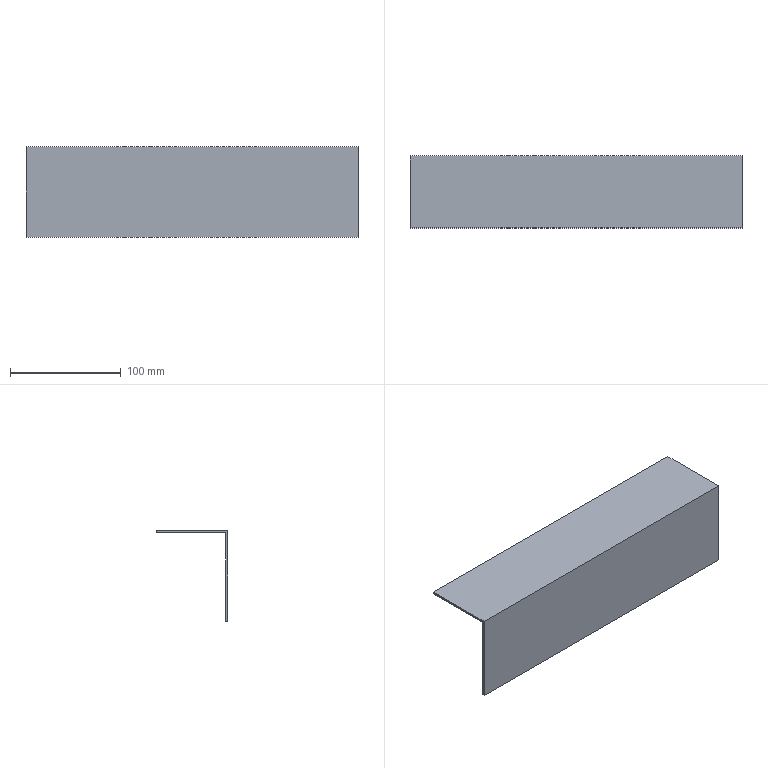Part | STEP file | MYT-A01-P21 | 1 solid | 8 faces | box 300 x 65 x 82 mm | volume 87000 mm3 | plane 8
STEP:
#1=CARTESIAN_POINT('',(-150.,-30.5,0.));
#2=VERTEX_POINT('',#1);
#3=CARTESIAN_POINT('',(150.,-30.5,0.));
#4=VERTEX_POINT('',#3);
#5=CARTESIAN_POINT('',(150.,-30.5,0.));
#6=DIRECTION('',(1.,0.,0.));
#7=VECTOR('',#6,1000.);
#8=LINE('',#5,#7);
#9=EDGE_CURVE('',#2,#4,#8,.T.);
#10=ORIENTED_EDGE('',*,*,#9,.F.);
#11=CARTESIAN_POINT('',(-150.,32.5,0.));
#12=VERTEX_POINT('',#11);
#13=CARTESIAN_POINT('',(-150.,32.5,0.));
#14=DIRECTION('',(0.,-1.,0.));
#15=VECTOR('',#14,1000.);
#16=LINE('',#13,#15);
#17=EDGE_CURVE('',#12,#2,#16,.T.);
#18=ORIENTED_EDGE('',*,*,#17,.F.);
#19=CARTESIAN_POINT('',(150.,32.5,0.));
#20=VERTEX_POINT('',#19);
#21=CARTESIAN_POINT('',(-150.,32.5,0.));
#22=DIRECTION('',(-1.,0.,0.));
#23=VECTOR('',#22,1000.);
#24=LINE('',#21,#23);
#25=EDGE_CURVE('',#20,#12,#24,.T.);
#26=ORIENTED_EDGE('',*,*,#25,.F.);
#27=CARTESIAN_POINT('',(150.,32.5,0.));
#28=DIRECTION('',(0.,1.,0.));
#29=VECTOR('',#28,1000.);
#30=LINE('',#27,#29);
#31=EDGE_CURVE('',#4,#20,#30,.T.);
#32=ORIENTED_EDGE('',*,*,#31,.F.);
#33=EDGE_LOOP('',(#10,#18,#26,#32));
#34=FACE_OUTER_BOUND('',#33,.T.);
#35=CARTESIAN_POINT('',(0.,0.,0.));
#36=DIRECTION('',(0.,0.,1.));
#37=DIRECTION('',(1.,0.,0.));
#38=AXIS2_PLACEMENT_3D('',#35,#36,#37);
#39=PLANE('',#38);
#40=ADVANCED_FACE('',(#34),#39,.F.);
#41=CARTESIAN_POINT('',(150.,-32.5,2.));
#42=VERTEX_POINT('',#41);
#43=CARTESIAN_POINT('',(150.,-32.5,-80.));
#44=VERTEX_POINT('',#43);
#45=CARTESIAN_POINT('',(150.,-32.5,2.));
#46=DIRECTION('',(0.,0.,-1.));
#47=VECTOR('',#46,1000.);
#48=LINE('',#45,#47);
#49=EDGE_CURVE('',#42,#44,#48,.T.);
#50=ORIENTED_EDGE('',*,*,#49,.T.);
#51=CARTESIAN_POINT('',(150.,-30.5,-80.));
#52=VERTEX_POINT('',#51);
#53=CARTESIAN_POINT('',(150.,-32.5,-80.));
#54=DIRECTION('',(0.,-1.,0.));
#55=VECTOR('',#54,1000.);
#56=LINE('',#53,#55);
#57=EDGE_CURVE('',#52,#44,#56,.T.);
#58=ORIENTED_EDGE('',*,*,#57,.F.);
#59=CARTESIAN_POINT('',(150.,-30.5,-80.));
#60=DIRECTION('',(0.,0.,1.));
#61=VECTOR('',#60,1000.);
#62=LINE('',#59,#61);
#63=EDGE_CURVE('',#52,#4,#62,.T.);
#64=ORIENTED_EDGE('',*,*,#63,.T.);
#65=ORIENTED_EDGE('',*,*,#31,.T.);
#66=CARTESIAN_POINT('',(150.,32.5,2.));
#67=VERTEX_POINT('',#66);
#68=CARTESIAN_POINT('',(150.,32.5,2.));
#69=DIRECTION('',(0.,0.,-1.));
#70=VECTOR('',#69,1000.);
#71=LINE('',#68,#70);
#72=EDGE_CURVE('',#67,#20,#71,.T.);
#73=ORIENTED_EDGE('',*,*,#72,.F.);
#74=CARTESIAN_POINT('',(150.,32.5,2.));
#75=DIRECTION('',(0.,1.,0.));
#76=VECTOR('',#75,1000.);
#77=LINE('',#74,#76);
#78=EDGE_CURVE('',#42,#67,#77,.T.);
#79=ORIENTED_EDGE('',*,*,#78,.F.);
#80=EDGE_LOOP('',(#50,#58,#64,#65,#73,#79));
#81=FACE_OUTER_BOUND('',#80,.T.);
#82=CARTESIAN_POINT('',(150.,32.5,2.));
#83=DIRECTION('',(-1.,0.,0.));
#84=DIRECTION('',(0.,0.,1.));
#85=AXIS2_PLACEMENT_3D('',#82,#83,#84);
#86=PLANE('',#85);
#87=ADVANCED_FACE('',(#81),#86,.F.);
#88=ORIENTED_EDGE('',*,*,#25,.T.);
#89=CARTESIAN_POINT('',(-150.,32.5,2.));
#90=VERTEX_POINT('',#89);
#91=CARTESIAN_POINT('',(-150.,32.5,2.));
#92=DIRECTION('',(0.,0.,-1.));
#93=VECTOR('',#92,1000.);
#94=LINE('',#91,#93);
#95=EDGE_CURVE('',#90,#12,#94,.T.);
#96=ORIENTED_EDGE('',*,*,#95,.F.);
#97=CARTESIAN_POINT('',(-150.,32.5,2.));
#98=DIRECTION('',(-1.,0.,0.));
#99=VECTOR('',#98,1000.);
#100=LINE('',#97,#99);
#101=EDGE_CURVE('',#67,#90,#100,.T.);
#102=ORIENTED_EDGE('',*,*,#101,.F.);
#103=ORIENTED_EDGE('',*,*,#72,.T.);
#104=EDGE_LOOP('',(#88,#96,#102,#103));
#105=FACE_OUTER_BOUND('',#104,.T.);
#106=CARTESIAN_POINT('',(-150.,32.5,2.));
#107=DIRECTION('',(0.,-1.,0.));
#108=DIRECTION('',(0.,0.,-1.));
#109=AXIS2_PLACEMENT_3D('',#106,#107,#108);
#110=PLANE('',#109);
#111=ADVANCED_FACE('',(#105),#110,.F.);
#112=ORIENTED_EDGE('',*,*,#17,.T.);
#113=CARTESIAN_POINT('',(-150.,-30.5,-80.));
#114=VERTEX_POINT('',#113);
#115=CARTESIAN_POINT('',(-150.,-30.5,-80.));
#116=DIRECTION('',(0.,0.,1.));
#117=VECTOR('',#116,1000.);
#118=LINE('',#115,#117);
#119=EDGE_CURVE('',#114,#2,#118,.T.);
#120=ORIENTED_EDGE('',*,*,#119,.F.);
#121=CARTESIAN_POINT('',(-150.,-32.5,-80.));
#122=VERTEX_POINT('',#121);
#123=CARTESIAN_POINT('',(-150.,-32.5,-80.));
#124=DIRECTION('',(0.,1.,0.));
#125=VECTOR('',#124,1000.);
#126=LINE('',#123,#125);
#127=EDGE_CURVE('',#122,#114,#126,.T.);
#128=ORIENTED_EDGE('',*,*,#127,.F.);
#129=CARTESIAN_POINT('',(-150.,-32.5,2.));
#130=VERTEX_POINT('',#129);
#131=CARTESIAN_POINT('',(-150.,-32.5,2.));
#132=DIRECTION('',(0.,0.,-1.));
#133=VECTOR('',#132,1000.);
#134=LINE('',#131,#133);
#135=EDGE_CURVE('',#130,#122,#134,.T.);
#136=ORIENTED_EDGE('',*,*,#135,.F.);
#137=CARTESIAN_POINT('',(-150.,32.5,2.));
#138=DIRECTION('',(0.,-1.,0.));
#139=VECTOR('',#138,1000.);
#140=LINE('',#137,#139);
#141=EDGE_CURVE('',#90,#130,#140,.T.);
#142=ORIENTED_EDGE('',*,*,#141,.F.);
#143=ORIENTED_EDGE('',*,*,#95,.T.);
#144=EDGE_LOOP('',(#112,#120,#128,#136,#142,#143));
#145=FACE_OUTER_BOUND('',#144,.T.);
#146=CARTESIAN_POINT('',(-150.,32.5,2.));
#147=DIRECTION('',(1.,0.,0.));
#148=DIRECTION('',(0.,0.,-1.));
#149=AXIS2_PLACEMENT_3D('',#146,#147,#148);
#150=PLANE('',#149);
#151=ADVANCED_FACE('',(#145),#150,.F.);
#152=ORIENTED_EDGE('',*,*,#135,.T.);
#153=CARTESIAN_POINT('',(150.,-32.5,-80.));
#154=DIRECTION('',(-1.,0.,0.));
#155=VECTOR('',#154,1000.);
#156=LINE('',#153,#155);
#157=EDGE_CURVE('',#44,#122,#156,.T.);
#158=ORIENTED_EDGE('',*,*,#157,.F.);
#159=ORIENTED_EDGE('',*,*,#49,.F.);
#160=CARTESIAN_POINT('',(-150.,-32.5,2.));
#161=DIRECTION('',(1.,0.,0.));
#162=VECTOR('',#161,1000.);
#163=LINE('',#160,#162);
#164=EDGE_CURVE('',#130,#42,#163,.T.);
#165=ORIENTED_EDGE('',*,*,#164,.F.);
#166=EDGE_LOOP('',(#152,#158,#159,#165));
#167=FACE_OUTER_BOUND('',#166,.T.);
#168=CARTESIAN_POINT('',(-150.,-32.5,2.));
#169=DIRECTION('',(0.,1.,0.));
#170=DIRECTION('',(0.,0.,1.));
#171=AXIS2_PLACEMENT_3D('',#168,#169,#170);
#172=PLANE('',#171);
#173=ADVANCED_FACE('',(#167),#172,.F.);
#174=ORIENTED_EDGE('',*,*,#78,.T.);
#175=ORIENTED_EDGE('',*,*,#101,.T.);
#176=ORIENTED_EDGE('',*,*,#141,.T.);
#177=ORIENTED_EDGE('',*,*,#164,.T.);
#178=EDGE_LOOP('',(#174,#175,#176,#177));
#179=FACE_OUTER_BOUND('',#178,.T.);
#180=CARTESIAN_POINT('',(0.,0.,2.));
#181=DIRECTION('',(0.,0.,1.));
#182=DIRECTION('',(1.,0.,0.));
#183=AXIS2_PLACEMENT_3D('',#180,#181,#182);
#184=PLANE('',#183);
#185=ADVANCED_FACE('',(#179),#184,.T.);
#186=ORIENTED_EDGE('',*,*,#9,.T.);
#187=ORIENTED_EDGE('',*,*,#63,.F.);
#188=CARTESIAN_POINT('',(150.,-30.5,-80.));
#189=DIRECTION('',(1.,0.,0.));
#190=VECTOR('',#189,1000.);
#191=LINE('',#188,#190);
#192=EDGE_CURVE('',#114,#52,#191,.T.);
#193=ORIENTED_EDGE('',*,*,#192,.F.);
#194=ORIENTED_EDGE('',*,*,#119,.T.);
#195=EDGE_LOOP('',(#186,#187,#193,#194));
#196=FACE_OUTER_BOUND('',#195,.T.);
#197=CARTESIAN_POINT('',(150.,-30.5,-80.));
#198=DIRECTION('',(0.,-1.,0.));
#199=DIRECTION('',(0.,0.,-1.));
#200=AXIS2_PLACEMENT_3D('',#197,#198,#199);
#201=PLANE('',#200);
#202=ADVANCED_FACE('',(#196),#201,.F.);
#203=ORIENTED_EDGE('',*,*,#57,.T.);
#204=ORIENTED_EDGE('',*,*,#157,.T.);
#205=ORIENTED_EDGE('',*,*,#127,.T.);
#206=ORIENTED_EDGE('',*,*,#192,.T.);
#207=EDGE_LOOP('',(#203,#204,#205,#206));
#208=FACE_OUTER_BOUND('',#207,.T.);
#209=CARTESIAN_POINT('',(0.,0.,-80.));
#210=DIRECTION('',(0.,0.,1.));
#211=DIRECTION('',(1.,0.,0.));
#212=AXIS2_PLACEMENT_3D('',#209,#210,#211);
#213=PLANE('',#212);
#214=ADVANCED_FACE('',(#208),#213,.F.);
#215=CLOSED_SHELL('',(#40,#87,#111,#151,#173,#185,#202,#214));
#216=MANIFOLD_SOLID_BREP('',#215);
#217=CARTESIAN_POINT('',(0.,0.,0.));
#218=DIRECTION('',(0.,0.,1.));
#219=DIRECTION('',(1.,0.,0.));
#220=AXIS2_PLACEMENT_3D('',#217,#218,#219);
#221=(LENGTH_UNIT()NAMED_UNIT(*)SI_UNIT(.MILLI.,.METRE.));
#222=UNCERTAINTY_MEASURE_WITH_UNIT(LENGTH_MEASURE(0.00001),#221,'','');
#223=(NAMED_UNIT(*)PLANE_ANGLE_UNIT()SI_UNIT($,.RADIAN.));
#224=(NAMED_UNIT(*)SI_UNIT($,.STERADIAN.)SOLID_ANGLE_UNIT());
#225=(GEOMETRIC_REPRESENTATION_CONTEXT(3)GLOBAL_UNCERTAINTY_ASSIGNED_CONTEXT((#222))GLOBAL_UNIT_ASSIGNED_CONTEXT((#221,#223,#224))REPRESENTATION_CONTEXT('',''));
#226=ADVANCED_BREP_SHAPE_REPRESENTATION('',(#216,#220),#225);